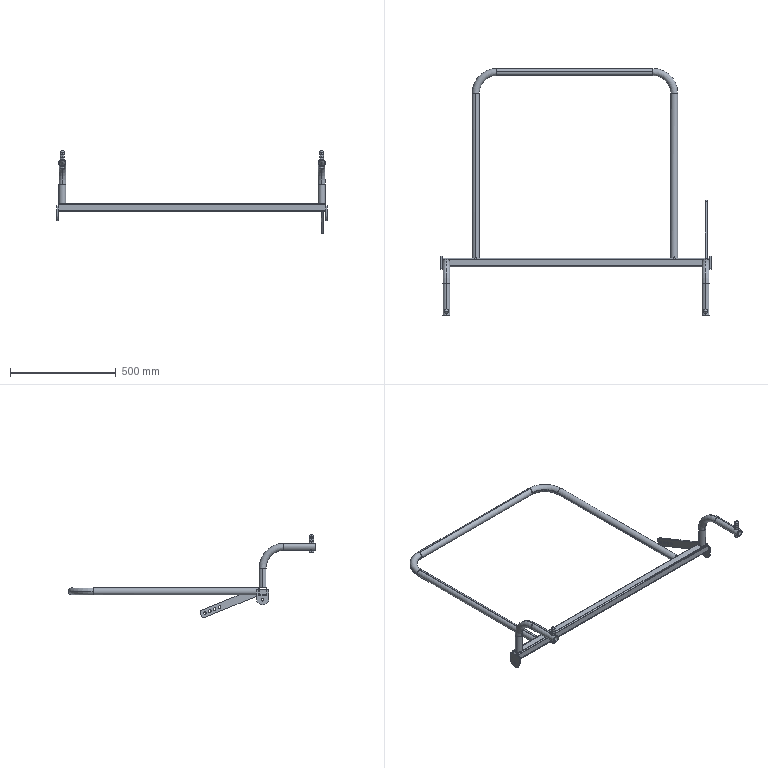Part | SolidWorks | features CompositeCurve 9, ReferencePattern 5, MirrorCompFeat 1 | 23 solids | 319 faces | box 1275 x 1167 x 393.469 mm | volume 1515109 mm3 | plane 122 | cone 96 | cylinder 81 | torus 16 | sphere 4 | commonest cylinder face diameters 12 x16 28.3 x14 33.3 x14 10.106 x12 13 x8 6 x4